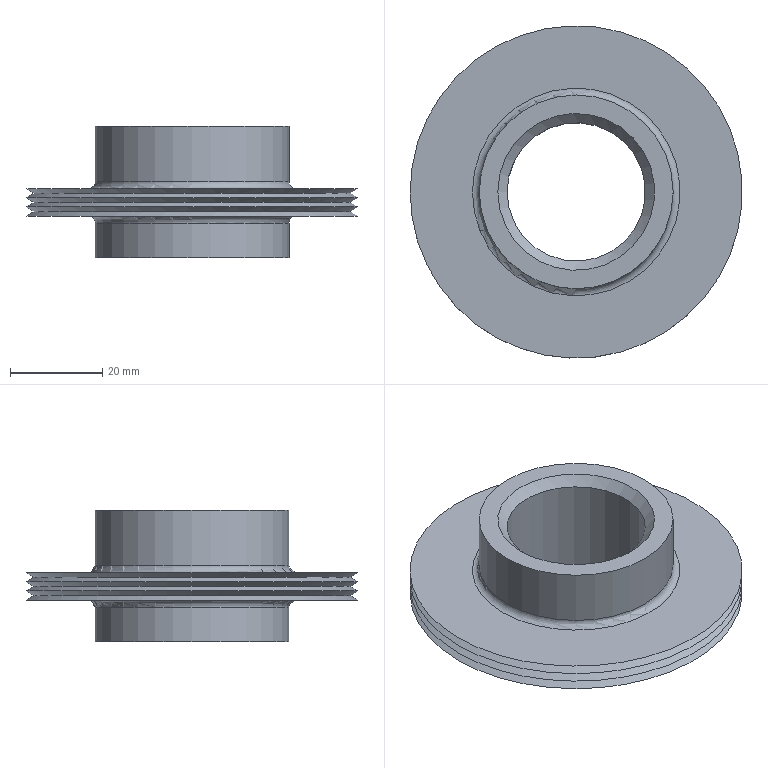Part | NX | features DATUM_CSYS 2, SKETCH 1, SWP104 1 | 1 solid | 17 faces | box 72 x 72 x 28.5 mm | volume 34035 mm3 | cone 8 | plane 4 | cylinder 3 | torus 2 | commonest cylinder face diameters 42 x2 30 x1
STEP:
#1=CARTESIAN_POINT('',(-36.,0.,9.));
#2=VERTEX_POINT('',#1);
#3=CARTESIAN_POINT('',(0.,0.,9.));
#4=DIRECTION('',(0.,0.,-1.));
#5=DIRECTION('',(-1.,0.,0.));
#6=AXIS2_PLACEMENT_3D('',#3,#4,#5);
#7=CIRCLE('',#6,36.);
#8=EDGE_CURVE('',#2,#2,#7,.T.);
#9=ORIENTED_EDGE('',*,*,#8,.F.);
#10=EDGE_LOOP('',(#9));
#11=FACE_BOUND('',#10,.T.);
#12=CARTESIAN_POINT('',(-34.268,0.,10.));
#13=VERTEX_POINT('',#12);
#14=CARTESIAN_POINT('',(0.,0.,10.));
#15=DIRECTION('',(0.,0.,-1.));
#16=DIRECTION('',(-1.,0.,0.));
#17=AXIS2_PLACEMENT_3D('',#14,#15,#16);
#18=CIRCLE('',#17,34.268);
#19=EDGE_CURVE('',#13,#13,#18,.T.);
#20=ORIENTED_EDGE('',*,*,#19,.T.);
#21=EDGE_LOOP('',(#20));
#22=FACE_BOUND('',#21,.T.);
#23=CARTESIAN_POINT('',(0.,0.,10.));
#24=DIRECTION('',(0.,0.,-1.));
#25=DIRECTION('',(-1.,0.,0.));
#26=AXIS2_PLACEMENT_3D('',#23,#24,#25);
#27=CONICAL_SURFACE('',#26,34.268,1.047);
#28=ADVANCED_FACE('',(#11,#22),#27,.T.);
#29=CARTESIAN_POINT('',(-22.5,0.,9.));
#30=VERTEX_POINT('',#29);
#31=CARTESIAN_POINT('',(0.,0.,9.));
#32=DIRECTION('',(0.,0.,-1.));
#33=DIRECTION('',(-1.,0.,0.));
#34=AXIS2_PLACEMENT_3D('',#31,#32,#33);
#35=CIRCLE('',#34,22.5);
#36=EDGE_CURVE('',#30,#30,#35,.T.);
#37=ORIENTED_EDGE('',*,*,#36,.F.);
#38=EDGE_LOOP('',(#37));
#39=FACE_BOUND('',#38,.T.);
#40=ORIENTED_EDGE('',*,*,#8,.T.);
#41=EDGE_LOOP('',(#40));
#42=FACE_BOUND('',#41,.T.);
#43=CARTESIAN_POINT('',(0.,-36.,9.));
#44=DIRECTION('',(0.,0.,1.));
#45=DIRECTION('',(1.,0.,0.));
#46=AXIS2_PLACEMENT_3D('',#43,#44,#45);
#47=PLANE('',#46);
#48=ADVANCED_FACE('',(#39,#42),#47,.F.);
#49=CARTESIAN_POINT('',(-21.,0.,7.5));
#50=VERTEX_POINT('',#49);
#51=CARTESIAN_POINT('',(0.,0.,7.5));
#52=DIRECTION('',(0.,0.,-1.));
#53=DIRECTION('',(-1.,0.,0.));
#54=AXIS2_PLACEMENT_3D('',#51,#52,#53);
#55=CIRCLE('',#54,21.);
#56=EDGE_CURVE('',#50,#50,#55,.T.);
#57=ORIENTED_EDGE('',*,*,#56,.F.);
#58=EDGE_LOOP('',(#57));
#59=FACE_BOUND('',#58,.T.);
#60=ORIENTED_EDGE('',*,*,#36,.T.);
#61=EDGE_LOOP('',(#60));
#62=FACE_BOUND('',#61,.T.);
#63=CARTESIAN_POINT('',(0.,0.,7.5));
#64=DIRECTION('',(0.,0.,-1.));
#65=DIRECTION('',(-1.,0.,0.));
#66=AXIS2_PLACEMENT_3D('',#63,#64,#65);
#67=TOROIDAL_SURFACE('',#66,22.5,1.5);
#68=ADVANCED_FACE('',(#59,#62),#67,.F.);
#69=CARTESIAN_POINT('',(-21.,0.,0.));
#70=VERTEX_POINT('',#69);
#71=CARTESIAN_POINT('',(0.,0.,0.));
#72=DIRECTION('',(0.,0.,-1.));
#73=DIRECTION('',(-1.,0.,0.));
#74=AXIS2_PLACEMENT_3D('',#71,#72,#73);
#75=CIRCLE('',#74,21.);
#76=EDGE_CURVE('',#70,#70,#75,.T.);
#77=ORIENTED_EDGE('',*,*,#76,.F.);
#78=EDGE_LOOP('',(#77));
#79=FACE_BOUND('',#78,.T.);
#80=ORIENTED_EDGE('',*,*,#56,.T.);
#81=EDGE_LOOP('',(#80));
#82=FACE_BOUND('',#81,.T.);
#83=CARTESIAN_POINT('',(0.,0.,0.));
#84=DIRECTION('',(0.,0.,-1.));
#85=DIRECTION('',(-1.,0.,0.));
#86=AXIS2_PLACEMENT_3D('',#83,#84,#85);
#87=CYLINDRICAL_SURFACE('',#86,21.);
#88=ADVANCED_FACE('',(#79,#82),#87,.T.);
#89=CARTESIAN_POINT('',(-17.,0.,0.));
#90=VERTEX_POINT('',#89);
#91=CARTESIAN_POINT('',(0.,0.,0.));
#92=DIRECTION('',(0.,0.,-1.));
#93=DIRECTION('',(-1.,0.,0.));
#94=AXIS2_PLACEMENT_3D('',#91,#92,#93);
#95=CIRCLE('',#94,17.);
#96=EDGE_CURVE('',#90,#90,#95,.T.);
#97=ORIENTED_EDGE('',*,*,#96,.F.);
#98=EDGE_LOOP('',(#97));
#99=FACE_BOUND('',#98,.T.);
#100=ORIENTED_EDGE('',*,*,#76,.T.);
#101=EDGE_LOOP('',(#100));
#102=FACE_BOUND('',#101,.T.);
#103=CARTESIAN_POINT('',(0.,-21.,0.));
#104=DIRECTION('',(0.,0.,1.));
#105=DIRECTION('',(1.,0.,0.));
#106=AXIS2_PLACEMENT_3D('',#103,#104,#105);
#107=PLANE('',#106);
#108=ADVANCED_FACE('',(#99,#102),#107,.F.);
#109=CARTESIAN_POINT('',(-15.,0.,2.));
#110=VERTEX_POINT('',#109);
#111=CARTESIAN_POINT('',(0.,0.,2.));
#112=DIRECTION('',(0.,0.,-1.));
#113=DIRECTION('',(-1.,0.,0.));
#114=AXIS2_PLACEMENT_3D('',#111,#112,#113);
#115=CIRCLE('',#114,15.);
#116=EDGE_CURVE('',#110,#110,#115,.T.);
#117=ORIENTED_EDGE('',*,*,#116,.F.);
#118=EDGE_LOOP('',(#117));
#119=FACE_BOUND('',#118,.T.);
#120=ORIENTED_EDGE('',*,*,#96,.T.);
#121=EDGE_LOOP('',(#120));
#122=FACE_BOUND('',#121,.T.);
#123=CARTESIAN_POINT('',(0.,0.,0.));
#124=DIRECTION('',(0.,0.,-1.));
#125=DIRECTION('',(-1.,0.,0.));
#126=AXIS2_PLACEMENT_3D('',#123,#124,#125);
#127=CONICAL_SURFACE('',#126,17.,0.7854);
#128=ADVANCED_FACE('',(#119,#122),#127,.F.);
#129=CARTESIAN_POINT('',(-15.,0.,26.5));
#130=VERTEX_POINT('',#129);
#131=CARTESIAN_POINT('',(0.,0.,26.5));
#132=DIRECTION('',(0.,0.,-1.));
#133=DIRECTION('',(-1.,0.,0.));
#134=AXIS2_PLACEMENT_3D('',#131,#132,#133);
#135=CIRCLE('',#134,15.);
#136=EDGE_CURVE('',#130,#130,#135,.T.);
#137=ORIENTED_EDGE('',*,*,#136,.F.);
#138=EDGE_LOOP('',(#137));
#139=FACE_BOUND('',#138,.T.);
#140=ORIENTED_EDGE('',*,*,#116,.T.);
#141=EDGE_LOOP('',(#140));
#142=FACE_BOUND('',#141,.T.);
#143=CARTESIAN_POINT('',(0.,0.,0.));
#144=DIRECTION('',(0.,0.,-1.));
#145=DIRECTION('',(-1.,0.,0.));
#146=AXIS2_PLACEMENT_3D('',#143,#144,#145);
#147=CYLINDRICAL_SURFACE('',#146,15.);
#148=ADVANCED_FACE('',(#139,#142),#147,.F.);
#149=CARTESIAN_POINT('',(-17.,0.,28.5));
#150=VERTEX_POINT('',#149);
#151=CARTESIAN_POINT('',(0.,0.,28.5));
#152=DIRECTION('',(0.,0.,-1.));
#153=DIRECTION('',(-1.,0.,0.));
#154=AXIS2_PLACEMENT_3D('',#151,#152,#153);
#155=CIRCLE('',#154,17.);
#156=EDGE_CURVE('',#150,#150,#155,.T.);
#157=ORIENTED_EDGE('',*,*,#156,.F.);
#158=EDGE_LOOP('',(#157));
#159=FACE_BOUND('',#158,.T.);
#160=ORIENTED_EDGE('',*,*,#136,.T.);
#161=EDGE_LOOP('',(#160));
#162=FACE_BOUND('',#161,.T.);
#163=CARTESIAN_POINT('',(0.,0.,26.5));
#164=DIRECTION('',(0.,0.,1.));
#165=DIRECTION('',(1.,0.,0.));
#166=AXIS2_PLACEMENT_3D('',#163,#164,#165);
#167=CONICAL_SURFACE('',#166,15.,0.7854);
#168=ADVANCED_FACE('',(#159,#162),#167,.F.);
#169=CARTESIAN_POINT('',(-21.,0.,28.5));
#170=VERTEX_POINT('',#169);
#171=CARTESIAN_POINT('',(0.,0.,28.5));
#172=DIRECTION('',(0.,0.,-1.));
#173=DIRECTION('',(-1.,0.,0.));
#174=AXIS2_PLACEMENT_3D('',#171,#172,#173);
#175=CIRCLE('',#174,21.);
#176=EDGE_CURVE('',#170,#170,#175,.T.);
#177=ORIENTED_EDGE('',*,*,#176,.F.);
#178=EDGE_LOOP('',(#177));
#179=FACE_BOUND('',#178,.T.);
#180=ORIENTED_EDGE('',*,*,#156,.T.);
#181=EDGE_LOOP('',(#180));
#182=FACE_BOUND('',#181,.T.);
#183=CARTESIAN_POINT('',(0.,-17.,28.5));
#184=DIRECTION('',(0.,0.,-1.));
#185=DIRECTION('',(-1.,0.,0.));
#186=AXIS2_PLACEMENT_3D('',#183,#184,#185);
#187=PLANE('',#186);
#188=ADVANCED_FACE('',(#179,#182),#187,.F.);
#189=CARTESIAN_POINT('',(-21.,0.,16.5));
#190=VERTEX_POINT('',#189);
#191=CARTESIAN_POINT('',(0.,0.,16.5));
#192=DIRECTION('',(0.,0.,-1.));
#193=DIRECTION('',(-1.,0.,0.));
#194=AXIS2_PLACEMENT_3D('',#191,#192,#193);
#195=CIRCLE('',#194,21.);
#196=EDGE_CURVE('',#190,#190,#195,.T.);
#197=ORIENTED_EDGE('',*,*,#196,.F.);
#198=EDGE_LOOP('',(#197));
#199=FACE_BOUND('',#198,.T.);
#200=ORIENTED_EDGE('',*,*,#176,.T.);
#201=EDGE_LOOP('',(#200));
#202=FACE_BOUND('',#201,.T.);
#203=CARTESIAN_POINT('',(0.,0.,0.));
#204=DIRECTION('',(0.,0.,-1.));
#205=DIRECTION('',(-1.,0.,0.));
#206=AXIS2_PLACEMENT_3D('',#203,#204,#205);
#207=CYLINDRICAL_SURFACE('',#206,21.);
#208=ADVANCED_FACE('',(#199,#202),#207,.T.);
#209=CARTESIAN_POINT('',(-22.5,0.,15.));
#210=VERTEX_POINT('',#209);
#211=CARTESIAN_POINT('',(0.,0.,15.));
#212=DIRECTION('',(0.,0.,-1.));
#213=DIRECTION('',(-1.,0.,0.));
#214=AXIS2_PLACEMENT_3D('',#211,#212,#213);
#215=CIRCLE('',#214,22.5);
#216=EDGE_CURVE('',#210,#210,#215,.T.);
#217=ORIENTED_EDGE('',*,*,#216,.F.);
#218=EDGE_LOOP('',(#217));
#219=FACE_BOUND('',#218,.T.);
#220=ORIENTED_EDGE('',*,*,#196,.T.);
#221=EDGE_LOOP('',(#220));
#222=FACE_BOUND('',#221,.T.);
#223=CARTESIAN_POINT('',(0.,0.,16.5));
#224=DIRECTION('',(0.,0.,-1.));
#225=DIRECTION('',(-1.,0.,0.));
#226=AXIS2_PLACEMENT_3D('',#223,#224,#225);
#227=TOROIDAL_SURFACE('',#226,22.5,1.5);
#228=ADVANCED_FACE('',(#219,#222),#227,.F.);
#229=CARTESIAN_POINT('',(-36.,0.,15.));
#230=VERTEX_POINT('',#229);
#231=CARTESIAN_POINT('',(0.,0.,15.));
#232=DIRECTION('',(0.,0.,-1.));
#233=DIRECTION('',(-1.,0.,0.));
#234=AXIS2_PLACEMENT_3D('',#231,#232,#233);
#235=CIRCLE('',#234,36.);
#236=EDGE_CURVE('',#230,#230,#235,.T.);
#237=ORIENTED_EDGE('',*,*,#236,.F.);
#238=EDGE_LOOP('',(#237));
#239=FACE_BOUND('',#238,.T.);
#240=ORIENTED_EDGE('',*,*,#216,.T.);
#241=EDGE_LOOP('',(#240));
#242=FACE_BOUND('',#241,.T.);
#243=CARTESIAN_POINT('',(0.,-22.5,15.));
#244=DIRECTION('',(0.,0.,-1.));
#245=DIRECTION('',(-1.,0.,0.));
#246=AXIS2_PLACEMENT_3D('',#243,#244,#245);
#247=PLANE('',#246);
#248=ADVANCED_FACE('',(#239,#242),#247,.F.);
#249=CARTESIAN_POINT('',(-34.268,0.,14.));
#250=VERTEX_POINT('',#249);
#251=CARTESIAN_POINT('',(0.,0.,14.));
#252=DIRECTION('',(0.,0.,-1.));
#253=DIRECTION('',(-1.,0.,0.));
#254=AXIS2_PLACEMENT_3D('',#251,#252,#253);
#255=CIRCLE('',#254,34.268);
#256=EDGE_CURVE('',#250,#250,#255,.T.);
#257=ORIENTED_EDGE('',*,*,#256,.F.);
#258=EDGE_LOOP('',(#257));
#259=FACE_BOUND('',#258,.T.);
#260=ORIENTED_EDGE('',*,*,#236,.T.);
#261=EDGE_LOOP('',(#260));
#262=FACE_BOUND('',#261,.T.);
#263=CARTESIAN_POINT('',(0.,0.,15.));
#264=DIRECTION('',(0.,0.,1.));
#265=DIRECTION('',(1.,0.,0.));
#266=AXIS2_PLACEMENT_3D('',#263,#264,#265);
#267=CONICAL_SURFACE('',#266,36.,1.047);
#268=ADVANCED_FACE('',(#259,#262),#267,.T.);
#269=CARTESIAN_POINT('',(-36.,0.,13.));
#270=VERTEX_POINT('',#269);
#271=CARTESIAN_POINT('',(0.,0.,13.));
#272=DIRECTION('',(0.,0.,-1.));
#273=DIRECTION('',(-1.,0.,0.));
#274=AXIS2_PLACEMENT_3D('',#271,#272,#273);
#275=CIRCLE('',#274,36.);
#276=EDGE_CURVE('',#270,#270,#275,.T.);
#277=ORIENTED_EDGE('',*,*,#276,.F.);
#278=EDGE_LOOP('',(#277));
#279=FACE_BOUND('',#278,.T.);
#280=ORIENTED_EDGE('',*,*,#256,.T.);
#281=EDGE_LOOP('',(#280));
#282=FACE_BOUND('',#281,.T.);
#283=CARTESIAN_POINT('',(0.,0.,14.));
#284=DIRECTION('',(0.,0.,-1.));
#285=DIRECTION('',(-1.,0.,0.));
#286=AXIS2_PLACEMENT_3D('',#283,#284,#285);
#287=CONICAL_SURFACE('',#286,34.268,1.047);
#288=ADVANCED_FACE('',(#279,#282),#287,.T.);
#289=CARTESIAN_POINT('',(-34.268,0.,12.));
#290=VERTEX_POINT('',#289);
#291=CARTESIAN_POINT('',(0.,0.,12.));
#292=DIRECTION('',(0.,0.,-1.));
#293=DIRECTION('',(-1.,0.,0.));
#294=AXIS2_PLACEMENT_3D('',#291,#292,#293);
#295=CIRCLE('',#294,34.268);
#296=EDGE_CURVE('',#290,#290,#295,.T.);
#297=ORIENTED_EDGE('',*,*,#296,.F.);
#298=EDGE_LOOP('',(#297));
#299=FACE_BOUND('',#298,.T.);
#300=ORIENTED_EDGE('',*,*,#276,.T.);
#301=EDGE_LOOP('',(#300));
#302=FACE_BOUND('',#301,.T.);
#303=CARTESIAN_POINT('',(0.,0.,13.));
#304=DIRECTION('',(0.,0.,1.));
#305=DIRECTION('',(1.,0.,0.));
#306=AXIS2_PLACEMENT_3D('',#303,#304,#305);
#307=CONICAL_SURFACE('',#306,36.,1.047);
#308=ADVANCED_FACE('',(#299,#302),#307,.T.);
#309=CARTESIAN_POINT('',(-36.,0.,11.));
#310=VERTEX_POINT('',#309);
#311=CARTESIAN_POINT('',(0.,0.,11.));
#312=DIRECTION('',(0.,0.,-1.));
#313=DIRECTION('',(-1.,0.,0.));
#314=AXIS2_PLACEMENT_3D('',#311,#312,#313);
#315=CIRCLE('',#314,36.);
#316=EDGE_CURVE('',#310,#310,#315,.T.);
#317=ORIENTED_EDGE('',*,*,#316,.F.);
#318=EDGE_LOOP('',(#317));
#319=FACE_BOUND('',#318,.T.);
#320=ORIENTED_EDGE('',*,*,#296,.T.);
#321=EDGE_LOOP('',(#320));
#322=FACE_BOUND('',#321,.T.);
#323=CARTESIAN_POINT('',(0.,0.,12.));
#324=DIRECTION('',(0.,0.,-1.));
#325=DIRECTION('',(-1.,0.,0.));
#326=AXIS2_PLACEMENT_3D('',#323,#324,#325);
#327=CONICAL_SURFACE('',#326,34.268,1.047);
#328=ADVANCED_FACE('',(#319,#322),#327,.T.);
#329=ORIENTED_EDGE('',*,*,#19,.F.);
#330=EDGE_LOOP('',(#329));
#331=FACE_BOUND('',#330,.T.);
#332=ORIENTED_EDGE('',*,*,#316,.T.);
#333=EDGE_LOOP('',(#332));
#334=FACE_BOUND('',#333,.T.);
#335=CARTESIAN_POINT('',(0.,0.,11.));
#336=DIRECTION('',(0.,0.,1.));
#337=DIRECTION('',(1.,0.,0.));
#338=AXIS2_PLACEMENT_3D('',#335,#336,#337);
#339=CONICAL_SURFACE('',#338,36.,1.047);
#340=ADVANCED_FACE('',(#331,#334),#339,.T.);
#341=CLOSED_SHELL('',(#28,#48,#68,#88,#108,#128,#148,#168,#188,#208,#228,#248,#268,#288,#308,#328,#340));
#342=MANIFOLD_SOLID_BREP('',#341);
#343=(LENGTH_UNIT()NAMED_UNIT(*)SI_UNIT(.MILLI.,.METRE.));
#344=UNCERTAINTY_MEASURE_WITH_UNIT(LENGTH_MEASURE(0.00001),#343,'','');
#345=(NAMED_UNIT(*)PLANE_ANGLE_UNIT()SI_UNIT($,.RADIAN.));
#346=(NAMED_UNIT(*)SI_UNIT($,.STERADIAN.)SOLID_ANGLE_UNIT());
#347=(GEOMETRIC_REPRESENTATION_CONTEXT(3)GLOBAL_UNCERTAINTY_ASSIGNED_CONTEXT((#344))GLOBAL_UNIT_ASSIGNED_CONTEXT((#343,#345,#346))REPRESENTATION_CONTEXT('',''));
#348=ADVANCED_BREP_SHAPE_REPRESENTATION('',(#342),#347);